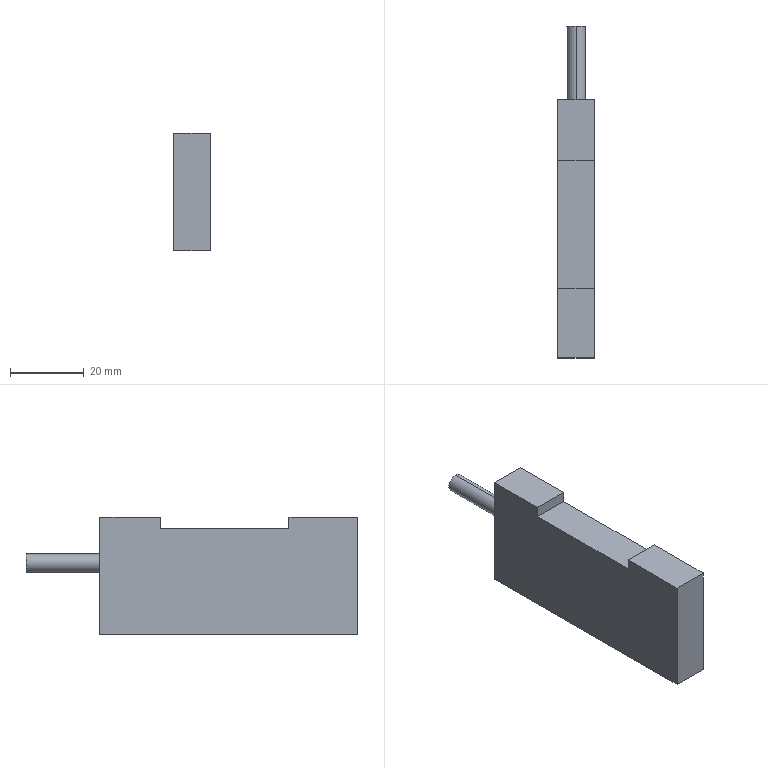Part | SolidWorks | features BaseBody 1, ICE 1 | 1 solid | 21 faces | box 10 x 90 x 32 mm | volume 21745 mm3 | plane 19 | cylinder 2 | commonest cylinder face diameters 5 x2
STEP:
#1=CARTESIAN_POINT('',(0.,0.,-15.));
#2=VERTEX_POINT('',#1);
#3=CARTESIAN_POINT('',(0.,0.,-10.));
#4=VERTEX_POINT('',#3);
#5=CARTESIAN_POINT('',(0.,0.,-12.5));
#6=DIRECTION('',(0.,-1.,0.));
#7=DIRECTION('',(0.,0.,1.));
#8=AXIS2_PLACEMENT_3D('',#5,#6,#7);
#9=CIRCLE('',#8,2.5);
#10=EDGE_CURVE('',#2,#4,#9,.T.);
#11=ORIENTED_EDGE('',*,*,#10,.F.);
#12=CARTESIAN_POINT('',(0.,20.,-15.));
#13=VERTEX_POINT('',#12);
#14=CARTESIAN_POINT('',(0.,0.,-15.));
#15=DIRECTION('',(0.,1.,0.));
#16=VECTOR('',#15,1000.);
#17=LINE('',#14,#16);
#18=EDGE_CURVE('',#2,#13,#17,.T.);
#19=ORIENTED_EDGE('',*,*,#18,.T.);
#20=CARTESIAN_POINT('',(0.,20.,-10.));
#21=VERTEX_POINT('',#20);
#22=CARTESIAN_POINT('',(0.,20.,-12.5));
#23=DIRECTION('',(0.,-1.,0.));
#24=DIRECTION('',(0.,0.,1.));
#25=AXIS2_PLACEMENT_3D('',#22,#23,#24);
#26=CIRCLE('',#25,2.5);
#27=EDGE_CURVE('',#13,#21,#26,.T.);
#28=ORIENTED_EDGE('',*,*,#27,.T.);
#29=CARTESIAN_POINT('',(0.,0.,-10.));
#30=DIRECTION('',(0.,1.,0.));
#31=VECTOR('',#30,1000.);
#32=LINE('',#29,#31);
#33=EDGE_CURVE('',#4,#21,#32,.T.);
#34=ORIENTED_EDGE('',*,*,#33,.F.);
#35=EDGE_LOOP('',(#11,#19,#28,#34));
#36=FACE_OUTER_BOUND('',#35,.T.);
#37=CARTESIAN_POINT('',(0.,0.,-12.5));
#38=DIRECTION('',(0.,1.,0.));
#39=DIRECTION('',(0.,0.,1.));
#40=AXIS2_PLACEMENT_3D('',#37,#38,#39);
#41=CYLINDRICAL_SURFACE('',#40,2.5);
#42=ADVANCED_FACE('',(#36),#41,.T.);
#43=CARTESIAN_POINT('',(-5.,-70.,-32.));
#44=VERTEX_POINT('',#43);
#45=CARTESIAN_POINT('',(-5.,0.,-32.));
#46=VERTEX_POINT('',#45);
#47=CARTESIAN_POINT('',(-5.,0.,-32.));
#48=DIRECTION('',(0.,1.,0.));
#49=VECTOR('',#48,1000.);
#50=LINE('',#47,#49);
#51=EDGE_CURVE('',#44,#46,#50,.T.);
#52=ORIENTED_EDGE('',*,*,#51,.F.);
#53=CARTESIAN_POINT('',(-5.,-70.,0.));
#54=VERTEX_POINT('',#53);
#55=CARTESIAN_POINT('',(-5.,-70.,0.));
#56=DIRECTION('',(0.,0.,-1.));
#57=VECTOR('',#56,1000.);
#58=LINE('',#55,#57);
#59=EDGE_CURVE('',#54,#44,#58,.T.);
#60=ORIENTED_EDGE('',*,*,#59,.F.);
#61=CARTESIAN_POINT('',(-5.,-51.3,0.));
#62=VERTEX_POINT('',#61);
#63=CARTESIAN_POINT('',(-5.,0.,0.));
#64=DIRECTION('',(0.,-1.,0.));
#65=VECTOR('',#64,1000.);
#66=LINE('',#63,#65);
#67=EDGE_CURVE('',#62,#54,#66,.T.);
#68=ORIENTED_EDGE('',*,*,#67,.F.);
#69=CARTESIAN_POINT('',(-5.,-51.3,-3.));
#70=VERTEX_POINT('',#69);
#71=CARTESIAN_POINT('',(-5.,-51.3,0.));
#72=DIRECTION('',(0.,0.,1.));
#73=VECTOR('',#72,1000.);
#74=LINE('',#71,#73);
#75=EDGE_CURVE('',#70,#62,#74,.T.);
#76=ORIENTED_EDGE('',*,*,#75,.F.);
#77=CARTESIAN_POINT('',(-5.,-16.5,-3.));
#78=VERTEX_POINT('',#77);
#79=CARTESIAN_POINT('',(-5.,0.,-3.));
#80=DIRECTION('',(0.,-1.,0.));
#81=VECTOR('',#80,1000.);
#82=LINE('',#79,#81);
#83=EDGE_CURVE('',#78,#70,#82,.T.);
#84=ORIENTED_EDGE('',*,*,#83,.F.);
#85=CARTESIAN_POINT('',(-5.,-16.5,0.));
#86=VERTEX_POINT('',#85);
#87=CARTESIAN_POINT('',(-5.,-16.5,0.));
#88=DIRECTION('',(0.,0.,-1.));
#89=VECTOR('',#88,1000.);
#90=LINE('',#87,#89);
#91=EDGE_CURVE('',#86,#78,#90,.T.);
#92=ORIENTED_EDGE('',*,*,#91,.F.);
#93=CARTESIAN_POINT('',(-5.,0.,0.));
#94=VERTEX_POINT('',#93);
#95=CARTESIAN_POINT('',(-5.,0.,0.));
#96=DIRECTION('',(0.,-1.,0.));
#97=VECTOR('',#96,1000.);
#98=LINE('',#95,#97);
#99=EDGE_CURVE('',#94,#86,#98,.T.);
#100=ORIENTED_EDGE('',*,*,#99,.F.);
#101=CARTESIAN_POINT('',(-5.,0.,0.));
#102=DIRECTION('',(0.,0.,1.));
#103=VECTOR('',#102,1000.);
#104=LINE('',#101,#103);
#105=EDGE_CURVE('',#46,#94,#104,.T.);
#106=ORIENTED_EDGE('',*,*,#105,.F.);
#107=EDGE_LOOP('',(#52,#60,#68,#76,#84,#92,#100,#106));
#108=FACE_OUTER_BOUND('',#107,.T.);
#109=CARTESIAN_POINT('',(-5.,0.,0.));
#110=DIRECTION('',(1.,0.,0.));
#111=DIRECTION('',(0.,0.,-1.));
#112=AXIS2_PLACEMENT_3D('',#109,#110,#111);
#113=PLANE('',#112);
#114=ADVANCED_FACE('',(#108),#113,.F.);
#115=CARTESIAN_POINT('',(5.,-70.,0.));
#116=VERTEX_POINT('',#115);
#117=CARTESIAN_POINT('',(5.,-51.3,0.));
#118=VERTEX_POINT('',#117);
#119=CARTESIAN_POINT('',(5.,0.,0.));
#120=DIRECTION('',(0.,1.,0.));
#121=VECTOR('',#120,1000.);
#122=LINE('',#119,#121);
#123=EDGE_CURVE('',#116,#118,#122,.T.);
#124=ORIENTED_EDGE('',*,*,#123,.T.);
#125=CARTESIAN_POINT('',(-5.,-51.3,0.));
#126=DIRECTION('',(-1.,0.,0.));
#127=VECTOR('',#126,1000.);
#128=LINE('',#125,#127);
#129=EDGE_CURVE('',#118,#62,#128,.T.);
#130=ORIENTED_EDGE('',*,*,#129,.T.);
#131=ORIENTED_EDGE('',*,*,#67,.T.);
#132=CARTESIAN_POINT('',(-5.,-70.,0.));
#133=DIRECTION('',(1.,0.,0.));
#134=VECTOR('',#133,1000.);
#135=LINE('',#132,#134);
#136=EDGE_CURVE('',#54,#116,#135,.T.);
#137=ORIENTED_EDGE('',*,*,#136,.T.);
#138=EDGE_LOOP('',(#124,#130,#131,#137));
#139=FACE_OUTER_BOUND('',#138,.T.);
#140=CARTESIAN_POINT('',(-5.,0.,0.));
#141=DIRECTION('',(0.,0.,1.));
#142=DIRECTION('',(1.,0.,0.));
#143=AXIS2_PLACEMENT_3D('',#140,#141,#142);
#144=PLANE('',#143);
#145=ADVANCED_FACE('',(#139),#144,.T.);
#146=CARTESIAN_POINT('',(5.,-51.3,-3.));
#147=VERTEX_POINT('',#146);
#148=CARTESIAN_POINT('',(5.,-51.3,0.));
#149=DIRECTION('',(0.,0.,1.));
#150=VECTOR('',#149,1000.);
#151=LINE('',#148,#150);
#152=EDGE_CURVE('',#147,#118,#151,.T.);
#153=ORIENTED_EDGE('',*,*,#152,.F.);
#154=CARTESIAN_POINT('',(5.,-51.3,-3.));
#155=DIRECTION('',(1.,0.,0.));
#156=VECTOR('',#155,1000.);
#157=LINE('',#154,#156);
#158=EDGE_CURVE('',#70,#147,#157,.T.);
#159=ORIENTED_EDGE('',*,*,#158,.F.);
#160=ORIENTED_EDGE('',*,*,#75,.T.);
#161=ORIENTED_EDGE('',*,*,#129,.F.);
#162=EDGE_LOOP('',(#153,#159,#160,#161));
#163=FACE_OUTER_BOUND('',#162,.T.);
#164=CARTESIAN_POINT('',(5.,-51.3,0.));
#165=DIRECTION('',(0.,-1.,0.));
#166=DIRECTION('',(0.,0.,-1.));
#167=AXIS2_PLACEMENT_3D('',#164,#165,#166);
#168=PLANE('',#167);
#169=ADVANCED_FACE('',(#163),#168,.F.);
#170=CARTESIAN_POINT('',(5.,-16.5,-3.));
#171=VERTEX_POINT('',#170);
#172=CARTESIAN_POINT('',(5.,-51.3,-3.));
#173=DIRECTION('',(0.,-1.,0.));
#174=VECTOR('',#173,1000.);
#175=LINE('',#172,#174);
#176=EDGE_CURVE('',#171,#147,#175,.T.);
#177=ORIENTED_EDGE('',*,*,#176,.F.);
#178=CARTESIAN_POINT('',(5.,-16.5,-3.));
#179=DIRECTION('',(1.,0.,0.));
#180=VECTOR('',#179,1000.);
#181=LINE('',#178,#180);
#182=EDGE_CURVE('',#78,#171,#181,.T.);
#183=ORIENTED_EDGE('',*,*,#182,.F.);
#184=ORIENTED_EDGE('',*,*,#83,.T.);
#185=ORIENTED_EDGE('',*,*,#158,.T.);
#186=EDGE_LOOP('',(#177,#183,#184,#185));
#187=FACE_OUTER_BOUND('',#186,.T.);
#188=CARTESIAN_POINT('',(5.,-51.3,-3.));
#189=DIRECTION('',(0.,0.,-1.));
#190=DIRECTION('',(-1.,0.,0.));
#191=AXIS2_PLACEMENT_3D('',#188,#189,#190);
#192=PLANE('',#191);
#193=ADVANCED_FACE('',(#187),#192,.F.);
#194=CARTESIAN_POINT('',(5.,-16.5,0.));
#195=VERTEX_POINT('',#194);
#196=CARTESIAN_POINT('',(5.,-16.5,-3.));
#197=DIRECTION('',(0.,0.,-1.));
#198=VECTOR('',#197,1000.);
#199=LINE('',#196,#198);
#200=EDGE_CURVE('',#195,#171,#199,.T.);
#201=ORIENTED_EDGE('',*,*,#200,.F.);
#202=CARTESIAN_POINT('',(5.,-16.5,0.));
#203=DIRECTION('',(1.,0.,0.));
#204=VECTOR('',#203,1000.);
#205=LINE('',#202,#204);
#206=EDGE_CURVE('',#86,#195,#205,.T.);
#207=ORIENTED_EDGE('',*,*,#206,.F.);
#208=ORIENTED_EDGE('',*,*,#91,.T.);
#209=ORIENTED_EDGE('',*,*,#182,.T.);
#210=EDGE_LOOP('',(#201,#207,#208,#209));
#211=FACE_OUTER_BOUND('',#210,.T.);
#212=CARTESIAN_POINT('',(5.,-16.5,-3.));
#213=DIRECTION('',(0.,1.,0.));
#214=DIRECTION('',(0.,0.,1.));
#215=AXIS2_PLACEMENT_3D('',#212,#213,#214);
#216=PLANE('',#215);
#217=ADVANCED_FACE('',(#211),#216,.F.);
#218=ORIENTED_EDGE('',*,*,#99,.T.);
#219=ORIENTED_EDGE('',*,*,#206,.T.);
#220=CARTESIAN_POINT('',(5.,0.,0.));
#221=VERTEX_POINT('',#220);
#222=CARTESIAN_POINT('',(5.,0.,0.));
#223=DIRECTION('',(0.,1.,0.));
#224=VECTOR('',#223,1000.);
#225=LINE('',#222,#224);
#226=EDGE_CURVE('',#195,#221,#225,.T.);
#227=ORIENTED_EDGE('',*,*,#226,.T.);
#228=CARTESIAN_POINT('',(-5.,0.,0.));
#229=DIRECTION('',(-1.,0.,0.));
#230=VECTOR('',#229,1000.);
#231=LINE('',#228,#230);
#232=EDGE_CURVE('',#221,#94,#231,.T.);
#233=ORIENTED_EDGE('',*,*,#232,.T.);
#234=EDGE_LOOP('',(#218,#219,#227,#233));
#235=FACE_OUTER_BOUND('',#234,.T.);
#236=CARTESIAN_POINT('',(-5.,0.,0.));
#237=DIRECTION('',(0.,0.,1.));
#238=DIRECTION('',(1.,0.,0.));
#239=AXIS2_PLACEMENT_3D('',#236,#237,#238);
#240=PLANE('',#239);
#241=ADVANCED_FACE('',(#235),#240,.T.);
#242=CARTESIAN_POINT('',(0.,0.,-12.5));
#243=DIRECTION('',(0.,-1.,0.));
#244=DIRECTION('',(0.,0.,1.));
#245=AXIS2_PLACEMENT_3D('',#242,#243,#244);
#246=CIRCLE('',#245,2.5);
#247=EDGE_CURVE('',#4,#2,#246,.T.);
#248=ORIENTED_EDGE('',*,*,#247,.T.);
#249=ORIENTED_EDGE('',*,*,#10,.T.);
#250=EDGE_LOOP('',(#248,#249));
#251=FACE_BOUND('',#250,.T.);
#252=CARTESIAN_POINT('',(5.,0.,-32.));
#253=VERTEX_POINT('',#252);
#254=CARTESIAN_POINT('',(-5.,0.,-32.));
#255=DIRECTION('',(-1.,0.,0.));
#256=VECTOR('',#255,1000.);
#257=LINE('',#254,#256);
#258=EDGE_CURVE('',#253,#46,#257,.T.);
#259=ORIENTED_EDGE('',*,*,#258,.T.);
#260=ORIENTED_EDGE('',*,*,#105,.T.);
#261=ORIENTED_EDGE('',*,*,#232,.F.);
#262=CARTESIAN_POINT('',(5.,0.,-32.));
#263=DIRECTION('',(0.,0.,-1.));
#264=VECTOR('',#263,1000.);
#265=LINE('',#262,#264);
#266=EDGE_CURVE('',#221,#253,#265,.T.);
#267=ORIENTED_EDGE('',*,*,#266,.T.);
#268=EDGE_LOOP('',(#259,#260,#261,#267));
#269=FACE_OUTER_BOUND('',#268,.T.);
#270=CARTESIAN_POINT('',(-5.,0.,-32.));
#271=DIRECTION('',(0.,1.,0.));
#272=DIRECTION('',(0.,0.,1.));
#273=AXIS2_PLACEMENT_3D('',#270,#271,#272);
#274=PLANE('',#273);
#275=ADVANCED_FACE('',(#251,#269),#274,.T.);
#276=CARTESIAN_POINT('',(-2.556,-13.979,-32.));
#277=VERTEX_POINT('',#276);
#278=CARTESIAN_POINT('',(-1.455,-13.979,-32.));
#279=VERTEX_POINT('',#278);
#280=CARTESIAN_POINT('',(-5.,-13.979,-32.));
#281=DIRECTION('',(1.,0.,0.));
#282=VECTOR('',#281,1000.);
#283=LINE('',#280,#282);
#284=EDGE_CURVE('',#277,#279,#283,.T.);
#285=ORIENTED_EDGE('',*,*,#284,.T.);
#286=CARTESIAN_POINT('',(-1.455,-18.304,-32.));
#287=VERTEX_POINT('',#286);
#288=CARTESIAN_POINT('',(-1.455,-70.,-32.));
#289=DIRECTION('',(0.,-1.,0.));
#290=VECTOR('',#289,1000.);
#291=LINE('',#288,#290);
#292=EDGE_CURVE('',#279,#287,#291,.T.);
#293=ORIENTED_EDGE('',*,*,#292,.T.);
#294=CARTESIAN_POINT('',(1.455,-18.304,-32.));
#295=VERTEX_POINT('',#294);
#296=CARTESIAN_POINT('',(-5.,-18.304,-32.));
#297=DIRECTION('',(1.,0.,0.));
#298=VECTOR('',#297,1000.);
#299=LINE('',#296,#298);
#300=EDGE_CURVE('',#287,#295,#299,.T.);
#301=ORIENTED_EDGE('',*,*,#300,.T.);
#302=CARTESIAN_POINT('',(1.455,-13.979,-32.));
#303=VERTEX_POINT('',#302);
#304=CARTESIAN_POINT('',(1.455,-70.,-32.));
#305=DIRECTION('',(0.,1.,0.));
#306=VECTOR('',#305,1000.);
#307=LINE('',#304,#306);
#308=EDGE_CURVE('',#295,#303,#307,.T.);
#309=ORIENTED_EDGE('',*,*,#308,.T.);
#310=CARTESIAN_POINT('',(2.556,-13.979,-32.));
#311=VERTEX_POINT('',#310);
#312=CARTESIAN_POINT('',(-5.,-13.979,-32.));
#313=DIRECTION('',(1.,0.,0.));
#314=VECTOR('',#313,1000.);
#315=LINE('',#312,#314);
#316=EDGE_CURVE('',#303,#311,#315,.T.);
#317=ORIENTED_EDGE('',*,*,#316,.T.);
#318=CARTESIAN_POINT('',(0.,-10.958,-32.));
#319=VERTEX_POINT('',#318);
#320=CARTESIAN_POINT('',(2.556,-13.979,-32.));
#321=DIRECTION('',(-0.6458,0.7635,0.));
#322=VECTOR('',#321,1000.);
#323=LINE('',#320,#322);
#324=EDGE_CURVE('',#311,#319,#323,.T.);
#325=ORIENTED_EDGE('',*,*,#324,.T.);
#326=CARTESIAN_POINT('',(0.,-10.958,-32.));
#327=DIRECTION('',(-0.6458,-0.7635,0.));
#328=VECTOR('',#327,1000.);
#329=LINE('',#326,#328);
#330=EDGE_CURVE('',#319,#277,#329,.T.);
#331=ORIENTED_EDGE('',*,*,#330,.T.);
#332=EDGE_LOOP('',(#285,#293,#301,#309,#317,#325,#331));
#333=FACE_BOUND('',#332,.T.);
#334=CARTESIAN_POINT('',(5.,-70.,-32.));
#335=VERTEX_POINT('',#334);
#336=CARTESIAN_POINT('',(-5.,-70.,-32.));
#337=DIRECTION('',(-1.,0.,0.));
#338=VECTOR('',#337,1000.);
#339=LINE('',#336,#338);
#340=EDGE_CURVE('',#335,#44,#339,.T.);
#341=ORIENTED_EDGE('',*,*,#340,.T.);
#342=ORIENTED_EDGE('',*,*,#51,.T.);
#343=ORIENTED_EDGE('',*,*,#258,.F.);
#344=CARTESIAN_POINT('',(5.,-70.,-32.));
#345=DIRECTION('',(0.,-1.,0.));
#346=VECTOR('',#345,1000.);
#347=LINE('',#344,#346);
#348=EDGE_CURVE('',#253,#335,#347,.T.);
#349=ORIENTED_EDGE('',*,*,#348,.T.);
#350=EDGE_LOOP('',(#341,#342,#343,#349));
#351=FACE_OUTER_BOUND('',#350,.T.);
#352=CARTESIAN_POINT('',(-5.,-70.,-32.));
#353=DIRECTION('',(0.,0.,-1.));
#354=DIRECTION('',(-1.,0.,0.));
#355=AXIS2_PLACEMENT_3D('',#352,#353,#354);
#356=PLANE('',#355);
#357=ADVANCED_FACE('',(#333,#351),#356,.T.);
#358=ORIENTED_EDGE('',*,*,#59,.T.);
#359=ORIENTED_EDGE('',*,*,#340,.F.);
#360=CARTESIAN_POINT('',(5.,-70.,0.));
#361=DIRECTION('',(0.,0.,1.));
#362=VECTOR('',#361,1000.);
#363=LINE('',#360,#362);
#364=EDGE_CURVE('',#335,#116,#363,.T.);
#365=ORIENTED_EDGE('',*,*,#364,.T.);
#366=ORIENTED_EDGE('',*,*,#136,.F.);
#367=EDGE_LOOP('',(#358,#359,#365,#366));
#368=FACE_OUTER_BOUND('',#367,.T.);
#369=CARTESIAN_POINT('',(-5.,-70.,0.));
#370=DIRECTION('',(0.,-1.,0.));
#371=DIRECTION('',(0.,0.,-1.));
#372=AXIS2_PLACEMENT_3D('',#369,#370,#371);
#373=PLANE('',#372);
#374=ADVANCED_FACE('',(#368),#373,.T.);
#375=ORIENTED_EDGE('',*,*,#364,.F.);
#376=ORIENTED_EDGE('',*,*,#348,.F.);
#377=ORIENTED_EDGE('',*,*,#266,.F.);
#378=ORIENTED_EDGE('',*,*,#226,.F.);
#379=ORIENTED_EDGE('',*,*,#200,.T.);
#380=ORIENTED_EDGE('',*,*,#176,.T.);
#381=ORIENTED_EDGE('',*,*,#152,.T.);
#382=ORIENTED_EDGE('',*,*,#123,.F.);
#383=EDGE_LOOP('',(#375,#376,#377,#378,#379,#380,#381,#382));
#384=FACE_OUTER_BOUND('',#383,.T.);
#385=CARTESIAN_POINT('',(5.,0.,0.));
#386=DIRECTION('',(1.,0.,0.));
#387=DIRECTION('',(0.,0.,-1.));
#388=AXIS2_PLACEMENT_3D('',#385,#386,#387);
#389=PLANE('',#388);
#390=ADVANCED_FACE('',(#384),#389,.T.);
#391=ORIENTED_EDGE('',*,*,#18,.F.);
#392=ORIENTED_EDGE('',*,*,#247,.F.);
#393=ORIENTED_EDGE('',*,*,#33,.T.);
#394=CARTESIAN_POINT('',(0.,20.,-12.5));
#395=DIRECTION('',(0.,-1.,0.));
#396=DIRECTION('',(0.,0.,1.));
#397=AXIS2_PLACEMENT_3D('',#394,#395,#396);
#398=CIRCLE('',#397,2.5);
#399=EDGE_CURVE('',#21,#13,#398,.T.);
#400=ORIENTED_EDGE('',*,*,#399,.T.);
#401=EDGE_LOOP('',(#391,#392,#393,#400));
#402=FACE_OUTER_BOUND('',#401,.T.);
#403=CARTESIAN_POINT('',(0.,0.,-12.5));
#404=DIRECTION('',(0.,1.,0.));
#405=DIRECTION('',(0.,0.,1.));
#406=AXIS2_PLACEMENT_3D('',#403,#404,#405);
#407=CYLINDRICAL_SURFACE('',#406,2.5);
#408=ADVANCED_FACE('',(#402),#407,.T.);
#409=CARTESIAN_POINT('',(-1.455,-18.304,-31.8));
#410=VERTEX_POINT('',#409);
#411=CARTESIAN_POINT('',(-1.455,-13.979,-31.8));
#412=VERTEX_POINT('',#411);
#413=CARTESIAN_POINT('',(-1.455,-18.304,-31.8));
#414=DIRECTION('',(0.,1.,0.));
#415=VECTOR('',#414,1000.);
#416=LINE('',#413,#415);
#417=EDGE_CURVE('',#410,#412,#416,.T.);
#418=ORIENTED_EDGE('',*,*,#417,.F.);
#419=CARTESIAN_POINT('',(-1.455,-18.304,-32.));
#420=DIRECTION('',(0.,0.,1.));
#421=VECTOR('',#420,1000.);
#422=LINE('',#419,#421);
#423=EDGE_CURVE('',#287,#410,#422,.T.);
#424=ORIENTED_EDGE('',*,*,#423,.F.);
#425=ORIENTED_EDGE('',*,*,#292,.F.);
#426=CARTESIAN_POINT('',(-1.455,-13.979,-32.));
#427=DIRECTION('',(0.,0.,-1.));
#428=VECTOR('',#427,1000.);
#429=LINE('',#426,#428);
#430=EDGE_CURVE('',#412,#279,#429,.T.);
#431=ORIENTED_EDGE('',*,*,#430,.F.);
#432=EDGE_LOOP('',(#418,#424,#425,#431));
#433=FACE_OUTER_BOUND('',#432,.T.);
#434=CARTESIAN_POINT('',(-1.455,-18.304,-32.));
#435=DIRECTION('',(-1.,0.,0.));
#436=DIRECTION('',(0.,0.,1.));
#437=AXIS2_PLACEMENT_3D('',#434,#435,#436);
#438=PLANE('',#437);
#439=ADVANCED_FACE('',(#433),#438,.F.);
#440=CARTESIAN_POINT('',(-2.556,-13.979,-31.8));
#441=VERTEX_POINT('',#440);
#442=CARTESIAN_POINT('',(-1.455,-13.979,-31.8));
#443=DIRECTION('',(-1.,0.,0.));
#444=VECTOR('',#443,1000.);
#445=LINE('',#442,#444);
#446=EDGE_CURVE('',#412,#441,#445,.T.);
#447=ORIENTED_EDGE('',*,*,#446,.F.);
#448=ORIENTED_EDGE('',*,*,#430,.T.);
#449=ORIENTED_EDGE('',*,*,#284,.F.);
#450=CARTESIAN_POINT('',(-2.556,-13.979,-32.));
#451=DIRECTION('',(0.,0.,-1.));
#452=VECTOR('',#451,1000.);
#453=LINE('',#450,#452);
#454=EDGE_CURVE('',#441,#277,#453,.T.);
#455=ORIENTED_EDGE('',*,*,#454,.F.);
#456=EDGE_LOOP('',(#447,#448,#449,#455));
#457=FACE_OUTER_BOUND('',#456,.T.);
#458=CARTESIAN_POINT('',(-1.455,-13.979,-32.));
#459=DIRECTION('',(0.,-1.,0.));
#460=DIRECTION('',(0.,0.,-1.));
#461=AXIS2_PLACEMENT_3D('',#458,#459,#460);
#462=PLANE('',#461);
#463=ADVANCED_FACE('',(#457),#462,.F.);
#464=CARTESIAN_POINT('',(0.,-10.958,-31.8));
#465=VERTEX_POINT('',#464);
#466=CARTESIAN_POINT('',(-2.556,-13.979,-31.8));
#467=DIRECTION('',(0.6458,0.7635,0.));
#468=VECTOR('',#467,1000.);
#469=LINE('',#466,#468);
#470=EDGE_CURVE('',#441,#465,#469,.T.);
#471=ORIENTED_EDGE('',*,*,#470,.F.);
#472=ORIENTED_EDGE('',*,*,#454,.T.);
#473=ORIENTED_EDGE('',*,*,#330,.F.);
#474=CARTESIAN_POINT('',(0.,-10.958,-32.));
#475=DIRECTION('',(0.,0.,-1.));
#476=VECTOR('',#475,1000.);
#477=LINE('',#474,#476);
#478=EDGE_CURVE('',#465,#319,#477,.T.);
#479=ORIENTED_EDGE('',*,*,#478,.F.);
#480=EDGE_LOOP('',(#471,#472,#473,#479));
#481=FACE_OUTER_BOUND('',#480,.T.);
#482=CARTESIAN_POINT('',(-2.556,-13.979,-32.));
#483=DIRECTION('',(-0.7635,0.6458,0.));
#484=DIRECTION('',(-0.6458,-0.7635,0.));
#485=AXIS2_PLACEMENT_3D('',#482,#483,#484);
#486=PLANE('',#485);
#487=ADVANCED_FACE('',(#481),#486,.F.);
#488=CARTESIAN_POINT('',(2.556,-13.979,-31.8));
#489=VERTEX_POINT('',#488);
#490=CARTESIAN_POINT('',(0.,-10.958,-31.8));
#491=DIRECTION('',(0.6458,-0.7635,0.));
#492=VECTOR('',#491,1000.);
#493=LINE('',#490,#492);
#494=EDGE_CURVE('',#465,#489,#493,.T.);
#495=ORIENTED_EDGE('',*,*,#494,.F.);
#496=ORIENTED_EDGE('',*,*,#478,.T.);
#497=ORIENTED_EDGE('',*,*,#324,.F.);
#498=CARTESIAN_POINT('',(2.556,-13.979,-32.));
#499=DIRECTION('',(0.,0.,-1.));
#500=VECTOR('',#499,1000.);
#501=LINE('',#498,#500);
#502=EDGE_CURVE('',#489,#311,#501,.T.);
#503=ORIENTED_EDGE('',*,*,#502,.F.);
#504=EDGE_LOOP('',(#495,#496,#497,#503));
#505=FACE_OUTER_BOUND('',#504,.T.);
#506=CARTESIAN_POINT('',(0.,-10.958,-32.));
#507=DIRECTION('',(0.7635,0.6458,0.));
#508=DIRECTION('',(-0.6458,0.7635,0.));
#509=AXIS2_PLACEMENT_3D('',#506,#507,#508);
#510=PLANE('',#509);
#511=ADVANCED_FACE('',(#505),#510,.F.);
#512=CARTESIAN_POINT('',(1.455,-13.979,-31.8));
#513=VERTEX_POINT('',#512);
#514=CARTESIAN_POINT('',(2.556,-13.979,-31.8));
#515=DIRECTION('',(-1.,0.,0.));
#516=VECTOR('',#515,1000.);
#517=LINE('',#514,#516);
#518=EDGE_CURVE('',#489,#513,#517,.T.);
#519=ORIENTED_EDGE('',*,*,#518,.F.);
#520=ORIENTED_EDGE('',*,*,#502,.T.);
#521=ORIENTED_EDGE('',*,*,#316,.F.);
#522=CARTESIAN_POINT('',(1.455,-13.979,-32.));
#523=DIRECTION('',(0.,0.,-1.));
#524=VECTOR('',#523,1000.);
#525=LINE('',#522,#524);
#526=EDGE_CURVE('',#513,#303,#525,.T.);
#527=ORIENTED_EDGE('',*,*,#526,.F.);
#528=EDGE_LOOP('',(#519,#520,#521,#527));
#529=FACE_OUTER_BOUND('',#528,.T.);
#530=CARTESIAN_POINT('',(2.556,-13.979,-32.));
#531=DIRECTION('',(0.,-1.,0.));
#532=DIRECTION('',(0.,0.,-1.));
#533=AXIS2_PLACEMENT_3D('',#530,#531,#532);
#534=PLANE('',#533);
#535=ADVANCED_FACE('',(#529),#534,.F.);
#536=CARTESIAN_POINT('',(1.455,-18.304,-31.8));
#537=VERTEX_POINT('',#536);
#538=CARTESIAN_POINT('',(1.455,-13.979,-31.8));
#539=DIRECTION('',(0.,-1.,0.));
#540=VECTOR('',#539,1000.);
#541=LINE('',#538,#540);
#542=EDGE_CURVE('',#513,#537,#541,.T.);
#543=ORIENTED_EDGE('',*,*,#542,.F.);
#544=ORIENTED_EDGE('',*,*,#526,.T.);
#545=ORIENTED_EDGE('',*,*,#308,.F.);
#546=CARTESIAN_POINT('',(1.455,-18.304,-32.));
#547=DIRECTION('',(0.,0.,-1.));
#548=VECTOR('',#547,1000.);
#549=LINE('',#546,#548);
#550=EDGE_CURVE('',#537,#295,#549,.T.);
#551=ORIENTED_EDGE('',*,*,#550,.F.);
#552=EDGE_LOOP('',(#543,#544,#545,#551));
#553=FACE_OUTER_BOUND('',#552,.T.);
#554=CARTESIAN_POINT('',(1.455,-13.979,-32.));
#555=DIRECTION('',(1.,0.,0.));
#556=DIRECTION('',(0.,0.,-1.));
#557=AXIS2_PLACEMENT_3D('',#554,#555,#556);
#558=PLANE('',#557);
#559=ADVANCED_FACE('',(#553),#558,.F.);
#560=CARTESIAN_POINT('',(1.455,-18.304,-31.8));
#561=DIRECTION('',(-1.,0.,0.));
#562=VECTOR('',#561,1000.);
#563=LINE('',#560,#562);
#564=EDGE_CURVE('',#537,#410,#563,.T.);
#565=ORIENTED_EDGE('',*,*,#564,.F.);
#566=ORIENTED_EDGE('',*,*,#550,.T.);
#567=ORIENTED_EDGE('',*,*,#300,.F.);
#568=ORIENTED_EDGE('',*,*,#423,.T.);
#569=EDGE_LOOP('',(#565,#566,#567,#568));
#570=FACE_OUTER_BOUND('',#569,.T.);
#571=CARTESIAN_POINT('',(1.455,-18.304,-32.));
#572=DIRECTION('',(0.,-1.,0.));
#573=DIRECTION('',(0.,0.,-1.));
#574=AXIS2_PLACEMENT_3D('',#571,#572,#573);
#575=PLANE('',#574);
#576=ADVANCED_FACE('',(#570),#575,.F.);
#577=ORIENTED_EDGE('',*,*,#399,.F.);
#578=ORIENTED_EDGE('',*,*,#27,.F.);
#579=EDGE_LOOP('',(#577,#578));
#580=FACE_OUTER_BOUND('',#579,.T.);
#581=CARTESIAN_POINT('',(-5.,20.,0.));
#582=DIRECTION('',(0.,1.,0.));
#583=DIRECTION('',(0.,0.,1.));
#584=AXIS2_PLACEMENT_3D('',#581,#582,#583);
#585=PLANE('',#584);
#586=ADVANCED_FACE('',(#580),#585,.T.);
#587=ORIENTED_EDGE('',*,*,#564,.T.);
#588=ORIENTED_EDGE('',*,*,#417,.T.);
#589=ORIENTED_EDGE('',*,*,#446,.T.);
#590=ORIENTED_EDGE('',*,*,#470,.T.);
#591=ORIENTED_EDGE('',*,*,#494,.T.);
#592=ORIENTED_EDGE('',*,*,#518,.T.);
#593=ORIENTED_EDGE('',*,*,#542,.T.);
#594=EDGE_LOOP('',(#587,#588,#589,#590,#591,#592,#593));
#595=FACE_OUTER_BOUND('',#594,.T.);
#596=CARTESIAN_POINT('',(-5.,0.,-31.8));
#597=DIRECTION('',(0.,0.,-1.));
#598=DIRECTION('',(-1.,0.,0.));
#599=AXIS2_PLACEMENT_3D('',#596,#597,#598);
#600=PLANE('',#599);
#601=ADVANCED_FACE('',(#595),#600,.T.);
#602=CLOSED_SHELL('',(#42,#114,#145,#169,#193,#217,#241,#275,#357,#374,#390,#408,#439,#463,#487,#511,#535,#559,#576,#586,#601));
#603=MANIFOLD_SOLID_BREP('',#602);
#604=CARTESIAN_POINT('',(0.,0.,0.));
#605=DIRECTION('',(0.,0.,1.));
#606=DIRECTION('',(1.,0.,0.));
#607=AXIS2_PLACEMENT_3D('',#604,#605,#606);
#608=(LENGTH_UNIT()NAMED_UNIT(*)SI_UNIT(.MILLI.,.METRE.));
#609=UNCERTAINTY_MEASURE_WITH_UNIT(LENGTH_MEASURE(0.00001),#608,'','');
#610=(NAMED_UNIT(*)PLANE_ANGLE_UNIT()SI_UNIT($,.RADIAN.));
#611=(NAMED_UNIT(*)SI_UNIT($,.STERADIAN.)SOLID_ANGLE_UNIT());
#612=(GEOMETRIC_REPRESENTATION_CONTEXT(3)GLOBAL_UNCERTAINTY_ASSIGNED_CONTEXT((#609))GLOBAL_UNIT_ASSIGNED_CONTEXT((#608,#610,#611))REPRESENTATION_CONTEXT('',''));
#613=ADVANCED_BREP_SHAPE_REPRESENTATION('',(#603,#607),#612);